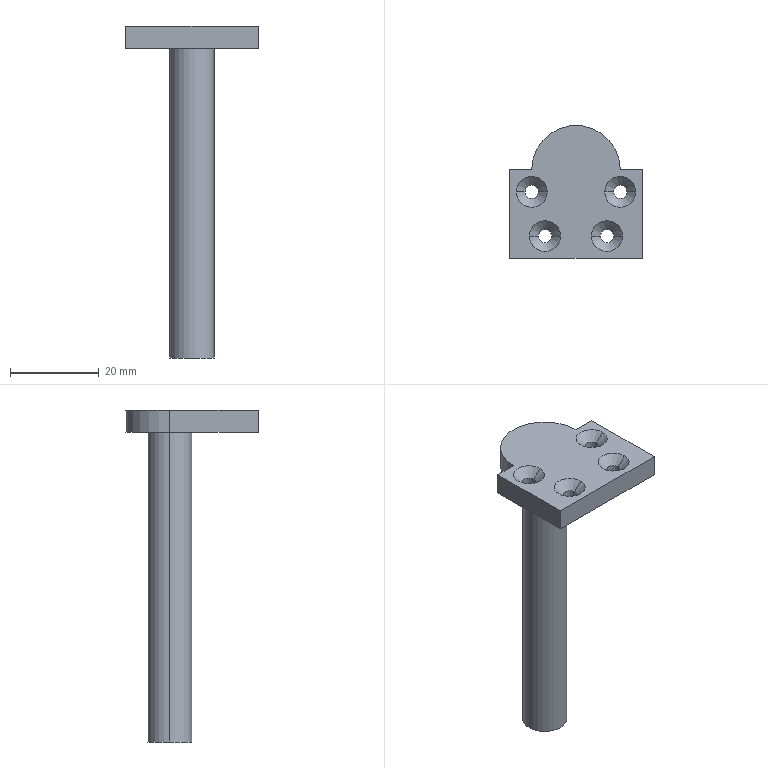Part | SolidWorks | features BaseBody 1 | 1 solid | 27 faces | box 30 x 30 x 75 mm | volume 9033 mm3 | cylinder 11 | cone 8 | plane 8 | commonest cylinder face diameters 3 x8 10 x2 20 x1
STEP:
#1=CARTESIAN_POINT('',(8.5,-5.,-2.));
#2=VERTEX_POINT('',#1);
#3=CARTESIAN_POINT('',(11.5,-5.,-2.));
#4=VERTEX_POINT('',#3);
#5=CARTESIAN_POINT('',(10.,-5.,-2.));
#6=DIRECTION('',(0.,0.,-1.));
#7=DIRECTION('',(-1.,0.,0.));
#8=AXIS2_PLACEMENT_3D('',#5,#6,#7);
#9=CIRCLE('',#8,1.5);
#10=EDGE_CURVE('',#2,#4,#9,.T.);
#11=ORIENTED_EDGE('',*,*,#10,.T.);
#12=CARTESIAN_POINT('',(13.5,-5.,0.));
#13=VERTEX_POINT('',#12);
#14=CARTESIAN_POINT('',(12.5,-5.,-1.));
#15=DIRECTION('',(0.7071,0.,0.7071));
#16=VECTOR('',#15,1000.);
#17=LINE('',#14,#16);
#18=EDGE_CURVE('',#4,#13,#17,.T.);
#19=ORIENTED_EDGE('',*,*,#18,.T.);
#20=CARTESIAN_POINT('',(6.5,-5.,0.));
#21=VERTEX_POINT('',#20);
#22=CARTESIAN_POINT('',(10.,-5.,0.));
#23=DIRECTION('',(0.,0.,1.));
#24=DIRECTION('',(-1.,0.,0.));
#25=AXIS2_PLACEMENT_3D('',#22,#23,#24);
#26=CIRCLE('',#25,3.5);
#27=EDGE_CURVE('',#13,#21,#26,.T.);
#28=ORIENTED_EDGE('',*,*,#27,.T.);
#29=CARTESIAN_POINT('',(7.5,-5.,-1.));
#30=DIRECTION('',(-0.7071,0.,0.7071));
#31=VECTOR('',#30,1000.);
#32=LINE('',#29,#31);
#33=EDGE_CURVE('',#2,#21,#32,.T.);
#34=ORIENTED_EDGE('',*,*,#33,.F.);
#35=EDGE_LOOP('',(#11,#19,#28,#34));
#36=FACE_OUTER_BOUND('',#35,.T.);
#37=CARTESIAN_POINT('',(10.,-5.,-1.));
#38=DIRECTION('',(0.,0.,1.));
#39=DIRECTION('',(-1.,0.,0.));
#40=AXIS2_PLACEMENT_3D('',#37,#38,#39);
#41=CONICAL_SURFACE('',#40,2.5,0.7854);
#42=ADVANCED_FACE('',(#36),#41,.F.);
#43=CARTESIAN_POINT('',(11.5,-5.,-5.));
#44=VERTEX_POINT('',#43);
#45=CARTESIAN_POINT('',(8.5,-5.,-5.));
#46=VERTEX_POINT('',#45);
#47=CARTESIAN_POINT('',(10.,-5.,-5.));
#48=DIRECTION('',(0.,0.,1.));
#49=DIRECTION('',(-1.,0.,0.));
#50=AXIS2_PLACEMENT_3D('',#47,#48,#49);
#51=CIRCLE('',#50,1.5);
#52=EDGE_CURVE('',#44,#46,#51,.T.);
#53=ORIENTED_EDGE('',*,*,#52,.F.);
#54=CARTESIAN_POINT('',(11.5,-5.,0.));
#55=DIRECTION('',(0.,0.,1.));
#56=VECTOR('',#55,1000.);
#57=LINE('',#54,#56);
#58=EDGE_CURVE('',#44,#4,#57,.T.);
#59=ORIENTED_EDGE('',*,*,#58,.T.);
#60=ORIENTED_EDGE('',*,*,#10,.F.);
#61=CARTESIAN_POINT('',(8.5,-5.,0.));
#62=DIRECTION('',(0.,0.,1.));
#63=VECTOR('',#62,1000.);
#64=LINE('',#61,#63);
#65=EDGE_CURVE('',#46,#2,#64,.T.);
#66=ORIENTED_EDGE('',*,*,#65,.F.);
#67=EDGE_LOOP('',(#53,#59,#60,#66));
#68=FACE_OUTER_BOUND('',#67,.T.);
#69=CARTESIAN_POINT('',(10.,-5.,0.));
#70=DIRECTION('',(0.,0.,1.));
#71=DIRECTION('',(-1.,0.,0.));
#72=AXIS2_PLACEMENT_3D('',#69,#70,#71);
#73=CYLINDRICAL_SURFACE('',#72,1.5);
#74=ADVANCED_FACE('',(#68),#73,.F.);
#75=CARTESIAN_POINT('',(5.5,-15.,-2.));
#76=VERTEX_POINT('',#75);
#77=CARTESIAN_POINT('',(8.5,-15.,-2.));
#78=VERTEX_POINT('',#77);
#79=CARTESIAN_POINT('',(7.,-15.,-2.));
#80=DIRECTION('',(0.,0.,-1.));
#81=DIRECTION('',(-1.,0.,0.));
#82=AXIS2_PLACEMENT_3D('',#79,#80,#81);
#83=CIRCLE('',#82,1.5);
#84=EDGE_CURVE('',#76,#78,#83,.T.);
#85=ORIENTED_EDGE('',*,*,#84,.T.);
#86=CARTESIAN_POINT('',(10.5,-15.,0.));
#87=VERTEX_POINT('',#86);
#88=CARTESIAN_POINT('',(9.5,-15.,-1.));
#89=DIRECTION('',(0.7071,0.,0.7071));
#90=VECTOR('',#89,1000.);
#91=LINE('',#88,#90);
#92=EDGE_CURVE('',#78,#87,#91,.T.);
#93=ORIENTED_EDGE('',*,*,#92,.T.);
#94=CARTESIAN_POINT('',(3.5,-15.,0.));
#95=VERTEX_POINT('',#94);
#96=CARTESIAN_POINT('',(7.,-15.,0.));
#97=DIRECTION('',(0.,0.,1.));
#98=DIRECTION('',(-1.,0.,0.));
#99=AXIS2_PLACEMENT_3D('',#96,#97,#98);
#100=CIRCLE('',#99,3.5);
#101=EDGE_CURVE('',#87,#95,#100,.T.);
#102=ORIENTED_EDGE('',*,*,#101,.T.);
#103=CARTESIAN_POINT('',(4.5,-15.,-1.));
#104=DIRECTION('',(-0.7071,0.,0.7071));
#105=VECTOR('',#104,1000.);
#106=LINE('',#103,#105);
#107=EDGE_CURVE('',#76,#95,#106,.T.);
#108=ORIENTED_EDGE('',*,*,#107,.F.);
#109=EDGE_LOOP('',(#85,#93,#102,#108));
#110=FACE_OUTER_BOUND('',#109,.T.);
#111=CARTESIAN_POINT('',(7.,-15.,-1.));
#112=DIRECTION('',(0.,0.,1.));
#113=DIRECTION('',(-1.,0.,0.));
#114=AXIS2_PLACEMENT_3D('',#111,#112,#113);
#115=CONICAL_SURFACE('',#114,2.5,0.7854);
#116=ADVANCED_FACE('',(#110),#115,.F.);
#117=CARTESIAN_POINT('',(8.5,-15.,-5.));
#118=VERTEX_POINT('',#117);
#119=CARTESIAN_POINT('',(5.5,-15.,-5.));
#120=VERTEX_POINT('',#119);
#121=CARTESIAN_POINT('',(7.,-15.,-5.));
#122=DIRECTION('',(0.,0.,1.));
#123=DIRECTION('',(-1.,0.,0.));
#124=AXIS2_PLACEMENT_3D('',#121,#122,#123);
#125=CIRCLE('',#124,1.5);
#126=EDGE_CURVE('',#118,#120,#125,.T.);
#127=ORIENTED_EDGE('',*,*,#126,.F.);
#128=CARTESIAN_POINT('',(8.5,-15.,0.));
#129=DIRECTION('',(0.,0.,1.));
#130=VECTOR('',#129,1000.);
#131=LINE('',#128,#130);
#132=EDGE_CURVE('',#118,#78,#131,.T.);
#133=ORIENTED_EDGE('',*,*,#132,.T.);
#134=ORIENTED_EDGE('',*,*,#84,.F.);
#135=CARTESIAN_POINT('',(5.5,-15.,0.));
#136=DIRECTION('',(0.,0.,1.));
#137=VECTOR('',#136,1000.);
#138=LINE('',#135,#137);
#139=EDGE_CURVE('',#120,#76,#138,.T.);
#140=ORIENTED_EDGE('',*,*,#139,.F.);
#141=EDGE_LOOP('',(#127,#133,#134,#140));
#142=FACE_OUTER_BOUND('',#141,.T.);
#143=CARTESIAN_POINT('',(7.,-15.,0.));
#144=DIRECTION('',(0.,0.,1.));
#145=DIRECTION('',(-1.,0.,0.));
#146=AXIS2_PLACEMENT_3D('',#143,#144,#145);
#147=CYLINDRICAL_SURFACE('',#146,1.5);
#148=ADVANCED_FACE('',(#142),#147,.F.);
#149=CARTESIAN_POINT('',(-8.5,-15.,-2.));
#150=VERTEX_POINT('',#149);
#151=CARTESIAN_POINT('',(-5.5,-15.,-2.));
#152=VERTEX_POINT('',#151);
#153=CARTESIAN_POINT('',(-7.,-15.,-2.));
#154=DIRECTION('',(0.,0.,-1.));
#155=DIRECTION('',(-1.,0.,0.));
#156=AXIS2_PLACEMENT_3D('',#153,#154,#155);
#157=CIRCLE('',#156,1.5);
#158=EDGE_CURVE('',#150,#152,#157,.T.);
#159=ORIENTED_EDGE('',*,*,#158,.T.);
#160=CARTESIAN_POINT('',(-3.5,-15.,0.));
#161=VERTEX_POINT('',#160);
#162=CARTESIAN_POINT('',(-4.5,-15.,-1.));
#163=DIRECTION('',(0.7071,0.,0.7071));
#164=VECTOR('',#163,1000.);
#165=LINE('',#162,#164);
#166=EDGE_CURVE('',#152,#161,#165,.T.);
#167=ORIENTED_EDGE('',*,*,#166,.T.);
#168=CARTESIAN_POINT('',(-10.5,-15.,0.));
#169=VERTEX_POINT('',#168);
#170=CARTESIAN_POINT('',(-7.,-15.,0.));
#171=DIRECTION('',(0.,0.,1.));
#172=DIRECTION('',(-1.,0.,0.));
#173=AXIS2_PLACEMENT_3D('',#170,#171,#172);
#174=CIRCLE('',#173,3.5);
#175=EDGE_CURVE('',#161,#169,#174,.T.);
#176=ORIENTED_EDGE('',*,*,#175,.T.);
#177=CARTESIAN_POINT('',(-9.5,-15.,-1.));
#178=DIRECTION('',(-0.7071,0.,0.7071));
#179=VECTOR('',#178,1000.);
#180=LINE('',#177,#179);
#181=EDGE_CURVE('',#150,#169,#180,.T.);
#182=ORIENTED_EDGE('',*,*,#181,.F.);
#183=EDGE_LOOP('',(#159,#167,#176,#182));
#184=FACE_OUTER_BOUND('',#183,.T.);
#185=CARTESIAN_POINT('',(-7.,-15.,-1.));
#186=DIRECTION('',(0.,0.,1.));
#187=DIRECTION('',(-1.,0.,0.));
#188=AXIS2_PLACEMENT_3D('',#185,#186,#187);
#189=CONICAL_SURFACE('',#188,2.5,0.7854);
#190=ADVANCED_FACE('',(#184),#189,.F.);
#191=CARTESIAN_POINT('',(-5.5,-15.,-5.));
#192=VERTEX_POINT('',#191);
#193=CARTESIAN_POINT('',(-8.5,-15.,-5.));
#194=VERTEX_POINT('',#193);
#195=CARTESIAN_POINT('',(-7.,-15.,-5.));
#196=DIRECTION('',(0.,0.,1.));
#197=DIRECTION('',(-1.,0.,0.));
#198=AXIS2_PLACEMENT_3D('',#195,#196,#197);
#199=CIRCLE('',#198,1.5);
#200=EDGE_CURVE('',#192,#194,#199,.T.);
#201=ORIENTED_EDGE('',*,*,#200,.F.);
#202=CARTESIAN_POINT('',(-5.5,-15.,0.));
#203=DIRECTION('',(0.,0.,1.));
#204=VECTOR('',#203,1000.);
#205=LINE('',#202,#204);
#206=EDGE_CURVE('',#192,#152,#205,.T.);
#207=ORIENTED_EDGE('',*,*,#206,.T.);
#208=ORIENTED_EDGE('',*,*,#158,.F.);
#209=CARTESIAN_POINT('',(-8.5,-15.,0.));
#210=DIRECTION('',(0.,0.,1.));
#211=VECTOR('',#210,1000.);
#212=LINE('',#209,#211);
#213=EDGE_CURVE('',#194,#150,#212,.T.);
#214=ORIENTED_EDGE('',*,*,#213,.F.);
#215=EDGE_LOOP('',(#201,#207,#208,#214));
#216=FACE_OUTER_BOUND('',#215,.T.);
#217=CARTESIAN_POINT('',(-7.,-15.,0.));
#218=DIRECTION('',(0.,0.,1.));
#219=DIRECTION('',(-1.,0.,0.));
#220=AXIS2_PLACEMENT_3D('',#217,#218,#219);
#221=CYLINDRICAL_SURFACE('',#220,1.5);
#222=ADVANCED_FACE('',(#216),#221,.F.);
#223=CARTESIAN_POINT('',(-11.5,-5.,-2.));
#224=VERTEX_POINT('',#223);
#225=CARTESIAN_POINT('',(-8.5,-5.,-2.));
#226=VERTEX_POINT('',#225);
#227=CARTESIAN_POINT('',(-10.,-5.,-2.));
#228=DIRECTION('',(0.,0.,-1.));
#229=DIRECTION('',(-1.,0.,0.));
#230=AXIS2_PLACEMENT_3D('',#227,#228,#229);
#231=CIRCLE('',#230,1.5);
#232=EDGE_CURVE('',#224,#226,#231,.T.);
#233=ORIENTED_EDGE('',*,*,#232,.T.);
#234=CARTESIAN_POINT('',(-6.5,-5.,0.));
#235=VERTEX_POINT('',#234);
#236=CARTESIAN_POINT('',(-7.5,-5.,-1.));
#237=DIRECTION('',(0.7071,0.,0.7071));
#238=VECTOR('',#237,1000.);
#239=LINE('',#236,#238);
#240=EDGE_CURVE('',#226,#235,#239,.T.);
#241=ORIENTED_EDGE('',*,*,#240,.T.);
#242=CARTESIAN_POINT('',(-13.5,-5.,0.));
#243=VERTEX_POINT('',#242);
#244=CARTESIAN_POINT('',(-10.,-5.,0.));
#245=DIRECTION('',(0.,0.,1.));
#246=DIRECTION('',(-1.,0.,0.));
#247=AXIS2_PLACEMENT_3D('',#244,#245,#246);
#248=CIRCLE('',#247,3.5);
#249=EDGE_CURVE('',#235,#243,#248,.T.);
#250=ORIENTED_EDGE('',*,*,#249,.T.);
#251=CARTESIAN_POINT('',(-12.5,-5.,-1.));
#252=DIRECTION('',(-0.7071,0.,0.7071));
#253=VECTOR('',#252,1000.);
#254=LINE('',#251,#253);
#255=EDGE_CURVE('',#224,#243,#254,.T.);
#256=ORIENTED_EDGE('',*,*,#255,.F.);
#257=EDGE_LOOP('',(#233,#241,#250,#256));
#258=FACE_OUTER_BOUND('',#257,.T.);
#259=CARTESIAN_POINT('',(-10.,-5.,-1.));
#260=DIRECTION('',(0.,0.,1.));
#261=DIRECTION('',(-1.,0.,0.));
#262=AXIS2_PLACEMENT_3D('',#259,#260,#261);
#263=CONICAL_SURFACE('',#262,2.5,0.7854);
#264=ADVANCED_FACE('',(#258),#263,.F.);
#265=CARTESIAN_POINT('',(-8.5,-5.,-5.));
#266=VERTEX_POINT('',#265);
#267=CARTESIAN_POINT('',(-11.5,-5.,-5.));
#268=VERTEX_POINT('',#267);
#269=CARTESIAN_POINT('',(-10.,-5.,-5.));
#270=DIRECTION('',(0.,0.,1.));
#271=DIRECTION('',(-1.,0.,0.));
#272=AXIS2_PLACEMENT_3D('',#269,#270,#271);
#273=CIRCLE('',#272,1.5);
#274=EDGE_CURVE('',#266,#268,#273,.T.);
#275=ORIENTED_EDGE('',*,*,#274,.F.);
#276=CARTESIAN_POINT('',(-8.5,-5.,0.));
#277=DIRECTION('',(0.,0.,1.));
#278=VECTOR('',#277,1000.);
#279=LINE('',#276,#278);
#280=EDGE_CURVE('',#266,#226,#279,.T.);
#281=ORIENTED_EDGE('',*,*,#280,.T.);
#282=ORIENTED_EDGE('',*,*,#232,.F.);
#283=CARTESIAN_POINT('',(-11.5,-5.,0.));
#284=DIRECTION('',(0.,0.,1.));
#285=VECTOR('',#284,1000.);
#286=LINE('',#283,#285);
#287=EDGE_CURVE('',#268,#224,#286,.T.);
#288=ORIENTED_EDGE('',*,*,#287,.F.);
#289=EDGE_LOOP('',(#275,#281,#282,#288));
#290=FACE_OUTER_BOUND('',#289,.T.);
#291=CARTESIAN_POINT('',(-10.,-5.,0.));
#292=DIRECTION('',(0.,0.,1.));
#293=DIRECTION('',(-1.,0.,0.));
#294=AXIS2_PLACEMENT_3D('',#291,#292,#293);
#295=CYLINDRICAL_SURFACE('',#294,1.5);
#296=ADVANCED_FACE('',(#290),#295,.F.);
#297=CARTESIAN_POINT('',(-5.,0.,-75.));
#298=VERTEX_POINT('',#297);
#299=CARTESIAN_POINT('',(5.,0.,-75.));
#300=VERTEX_POINT('',#299);
#301=CARTESIAN_POINT('',(0.,0.,-75.));
#302=DIRECTION('',(0.,0.,-1.));
#303=DIRECTION('',(1.,0.,0.));
#304=AXIS2_PLACEMENT_3D('',#301,#302,#303);
#305=CIRCLE('',#304,5.);
#306=EDGE_CURVE('',#298,#300,#305,.T.);
#307=ORIENTED_EDGE('',*,*,#306,.F.);
#308=CARTESIAN_POINT('',(-5.,0.,-5.));
#309=VERTEX_POINT('',#308);
#310=CARTESIAN_POINT('',(-5.,0.,-5.));
#311=DIRECTION('',(0.,0.,1.));
#312=VECTOR('',#311,1000.);
#313=LINE('',#310,#312);
#314=EDGE_CURVE('',#298,#309,#313,.T.);
#315=ORIENTED_EDGE('',*,*,#314,.T.);
#316=CARTESIAN_POINT('',(5.,0.,-5.));
#317=VERTEX_POINT('',#316);
#318=CARTESIAN_POINT('',(0.,0.,-5.));
#319=DIRECTION('',(0.,0.,1.));
#320=DIRECTION('',(1.,0.,0.));
#321=AXIS2_PLACEMENT_3D('',#318,#319,#320);
#322=CIRCLE('',#321,5.);
#323=EDGE_CURVE('',#317,#309,#322,.T.);
#324=ORIENTED_EDGE('',*,*,#323,.F.);
#325=CARTESIAN_POINT('',(5.,0.,-5.));
#326=DIRECTION('',(0.,0.,1.));
#327=VECTOR('',#326,1000.);
#328=LINE('',#325,#327);
#329=EDGE_CURVE('',#300,#317,#328,.T.);
#330=ORIENTED_EDGE('',*,*,#329,.F.);
#331=EDGE_LOOP('',(#307,#315,#324,#330));
#332=FACE_OUTER_BOUND('',#331,.T.);
#333=CARTESIAN_POINT('',(0.,0.,-5.));
#334=DIRECTION('',(0.,0.,1.));
#335=DIRECTION('',(1.,0.,0.));
#336=AXIS2_PLACEMENT_3D('',#333,#334,#335);
#337=CYLINDRICAL_SURFACE('',#336,5.);
#338=ADVANCED_FACE('',(#332),#337,.T.);
#339=CARTESIAN_POINT('',(7.,-15.,0.));
#340=DIRECTION('',(0.,0.,1.));
#341=DIRECTION('',(-1.,0.,0.));
#342=AXIS2_PLACEMENT_3D('',#339,#340,#341);
#343=CIRCLE('',#342,3.5);
#344=EDGE_CURVE('',#95,#87,#343,.T.);
#345=ORIENTED_EDGE('',*,*,#344,.F.);
#346=ORIENTED_EDGE('',*,*,#101,.F.);
#347=EDGE_LOOP('',(#345,#346));
#348=FACE_BOUND('',#347,.T.);
#349=CARTESIAN_POINT('',(-10.,-5.,0.));
#350=DIRECTION('',(0.,0.,1.));
#351=DIRECTION('',(-1.,0.,0.));
#352=AXIS2_PLACEMENT_3D('',#349,#350,#351);
#353=CIRCLE('',#352,3.5);
#354=EDGE_CURVE('',#243,#235,#353,.T.);
#355=ORIENTED_EDGE('',*,*,#354,.F.);
#356=ORIENTED_EDGE('',*,*,#249,.F.);
#357=EDGE_LOOP('',(#355,#356));
#358=FACE_BOUND('',#357,.T.);
#359=CARTESIAN_POINT('',(-7.,-15.,0.));
#360=DIRECTION('',(0.,0.,1.));
#361=DIRECTION('',(-1.,0.,0.));
#362=AXIS2_PLACEMENT_3D('',#359,#360,#361);
#363=CIRCLE('',#362,3.5);
#364=EDGE_CURVE('',#169,#161,#363,.T.);
#365=ORIENTED_EDGE('',*,*,#364,.F.);
#366=ORIENTED_EDGE('',*,*,#175,.F.);
#367=EDGE_LOOP('',(#365,#366));
#368=FACE_BOUND('',#367,.T.);
#369=CARTESIAN_POINT('',(10.,-5.,0.));
#370=DIRECTION('',(0.,0.,1.));
#371=DIRECTION('',(-1.,0.,0.));
#372=AXIS2_PLACEMENT_3D('',#369,#370,#371);
#373=CIRCLE('',#372,3.5);
#374=EDGE_CURVE('',#21,#13,#373,.T.);
#375=ORIENTED_EDGE('',*,*,#374,.F.);
#376=ORIENTED_EDGE('',*,*,#27,.F.);
#377=EDGE_LOOP('',(#375,#376));
#378=FACE_BOUND('',#377,.T.);
#379=CARTESIAN_POINT('',(10.,0.,0.));
#380=VERTEX_POINT('',#379);
#381=CARTESIAN_POINT('',(-10.,0.,0.));
#382=VERTEX_POINT('',#381);
#383=CARTESIAN_POINT('',(0.,0.,0.));
#384=DIRECTION('',(0.,0.,1.));
#385=DIRECTION('',(1.,0.,0.));
#386=AXIS2_PLACEMENT_3D('',#383,#384,#385);
#387=CIRCLE('',#386,10.);
#388=EDGE_CURVE('',#380,#382,#387,.T.);
#389=ORIENTED_EDGE('',*,*,#388,.T.);
#390=CARTESIAN_POINT('',(-15.,0.,0.));
#391=VERTEX_POINT('',#390);
#392=CARTESIAN_POINT('',(15.,0.,0.));
#393=DIRECTION('',(-1.,0.,0.));
#394=VECTOR('',#393,1000.);
#395=LINE('',#392,#394);
#396=EDGE_CURVE('',#382,#391,#395,.T.);
#397=ORIENTED_EDGE('',*,*,#396,.T.);
#398=CARTESIAN_POINT('',(-15.,-20.,0.));
#399=VERTEX_POINT('',#398);
#400=CARTESIAN_POINT('',(-15.,0.,0.));
#401=DIRECTION('',(0.,-1.,0.));
#402=VECTOR('',#401,1000.);
#403=LINE('',#400,#402);
#404=EDGE_CURVE('',#391,#399,#403,.T.);
#405=ORIENTED_EDGE('',*,*,#404,.T.);
#406=CARTESIAN_POINT('',(15.,-20.,0.));
#407=VERTEX_POINT('',#406);
#408=CARTESIAN_POINT('',(-15.,-20.,0.));
#409=DIRECTION('',(1.,0.,0.));
#410=VECTOR('',#409,1000.);
#411=LINE('',#408,#410);
#412=EDGE_CURVE('',#399,#407,#411,.T.);
#413=ORIENTED_EDGE('',*,*,#412,.T.);
#414=CARTESIAN_POINT('',(15.,0.,0.));
#415=VERTEX_POINT('',#414);
#416=CARTESIAN_POINT('',(15.,-20.,0.));
#417=DIRECTION('',(0.,1.,0.));
#418=VECTOR('',#417,1000.);
#419=LINE('',#416,#418);
#420=EDGE_CURVE('',#407,#415,#419,.T.);
#421=ORIENTED_EDGE('',*,*,#420,.T.);
#422=CARTESIAN_POINT('',(15.,0.,0.));
#423=DIRECTION('',(-1.,0.,0.));
#424=VECTOR('',#423,1000.);
#425=LINE('',#422,#424);
#426=EDGE_CURVE('',#415,#380,#425,.T.);
#427=ORIENTED_EDGE('',*,*,#426,.T.);
#428=EDGE_LOOP('',(#389,#397,#405,#413,#421,#427));
#429=FACE_OUTER_BOUND('',#428,.T.);
#430=CARTESIAN_POINT('',(0.,3.443,0.));
#431=DIRECTION('',(0.,0.,1.));
#432=DIRECTION('',(1.,0.,0.));
#433=AXIS2_PLACEMENT_3D('',#430,#431,#432);
#434=PLANE('',#433);
#435=ADVANCED_FACE('',(#348,#358,#368,#378,#429),#434,.T.);
#436=CARTESIAN_POINT('',(0.,0.,-75.));
#437=DIRECTION('',(0.,0.,-1.));
#438=DIRECTION('',(1.,0.,0.));
#439=AXIS2_PLACEMENT_3D('',#436,#437,#438);
#440=CIRCLE('',#439,5.);
#441=EDGE_CURVE('',#300,#298,#440,.T.);
#442=ORIENTED_EDGE('',*,*,#441,.T.);
#443=ORIENTED_EDGE('',*,*,#306,.T.);
#444=EDGE_LOOP('',(#442,#443));
#445=FACE_OUTER_BOUND('',#444,.T.);
#446=CARTESIAN_POINT('',(0.,0.,-75.));
#447=DIRECTION('',(0.,0.,1.));
#448=DIRECTION('',(1.,0.,0.));
#449=AXIS2_PLACEMENT_3D('',#446,#447,#448);
#450=PLANE('',#449);
#451=ADVANCED_FACE('',(#445),#450,.F.);
#452=CARTESIAN_POINT('',(-10.,0.,-5.));
#453=VERTEX_POINT('',#452);
#454=CARTESIAN_POINT('',(-10.,0.,0.));
#455=DIRECTION('',(0.,0.,-1.));
#456=VECTOR('',#455,1000.);
#457=LINE('',#454,#456);
#458=EDGE_CURVE('',#382,#453,#457,.T.);
#459=ORIENTED_EDGE('',*,*,#458,.T.);
#460=CARTESIAN_POINT('',(-15.,0.,-5.));
#461=VERTEX_POINT('',#460);
#462=CARTESIAN_POINT('',(15.,0.,-5.));
#463=DIRECTION('',(1.,0.,0.));
#464=VECTOR('',#463,1000.);
#465=LINE('',#462,#464);
#466=EDGE_CURVE('',#461,#453,#465,.T.);
#467=ORIENTED_EDGE('',*,*,#466,.F.);
#468=CARTESIAN_POINT('',(-15.,0.,0.));
#469=DIRECTION('',(0.,0.,-1.));
#470=VECTOR('',#469,1000.);
#471=LINE('',#468,#470);
#472=EDGE_CURVE('',#391,#461,#471,.T.);
#473=ORIENTED_EDGE('',*,*,#472,.F.);
#474=ORIENTED_EDGE('',*,*,#396,.F.);
#475=EDGE_LOOP('',(#459,#467,#473,#474));
#476=FACE_OUTER_BOUND('',#475,.T.);
#477=CARTESIAN_POINT('',(-15.,0.,0.));
#478=DIRECTION('',(0.,1.,0.));
#479=DIRECTION('',(1.,0.,0.));
#480=AXIS2_PLACEMENT_3D('',#477,#478,#479);
#481=PLANE('',#480);
#482=ADVANCED_FACE('',(#476),#481,.T.);
#483=CARTESIAN_POINT('',(10.,0.,-5.));
#484=VERTEX_POINT('',#483);
#485=CARTESIAN_POINT('',(10.,0.,0.));
#486=DIRECTION('',(0.,0.,-1.));
#487=VECTOR('',#486,1000.);
#488=LINE('',#485,#487);
#489=EDGE_CURVE('',#380,#484,#488,.T.);
#490=ORIENTED_EDGE('',*,*,#489,.F.);
#491=ORIENTED_EDGE('',*,*,#426,.F.);
#492=CARTESIAN_POINT('',(15.,0.,-5.));
#493=VERTEX_POINT('',#492);
#494=CARTESIAN_POINT('',(15.,0.,0.));
#495=DIRECTION('',(0.,0.,-1.));
#496=VECTOR('',#495,1000.);
#497=LINE('',#494,#496);
#498=EDGE_CURVE('',#415,#493,#497,.T.);
#499=ORIENTED_EDGE('',*,*,#498,.T.);
#500=CARTESIAN_POINT('',(15.,0.,-5.));
#501=DIRECTION('',(1.,0.,0.));
#502=VECTOR('',#501,1000.);
#503=LINE('',#500,#502);
#504=EDGE_CURVE('',#484,#493,#503,.T.);
#505=ORIENTED_EDGE('',*,*,#504,.F.);
#506=EDGE_LOOP('',(#490,#491,#499,#505));
#507=FACE_OUTER_BOUND('',#506,.T.);
#508=CARTESIAN_POINT('',(-15.,0.,0.));
#509=DIRECTION('',(0.,1.,0.));
#510=DIRECTION('',(1.,0.,0.));
#511=AXIS2_PLACEMENT_3D('',#508,#509,#510);
#512=PLANE('',#511);
#513=ADVANCED_FACE('',(#507),#512,.T.);
#514=ORIENTED_EDGE('',*,*,#412,.F.);
#515=CARTESIAN_POINT('',(-15.,-20.,-5.));
#516=VERTEX_POINT('',#515);
#517=CARTESIAN_POINT('',(-15.,-20.,0.));
#518=DIRECTION('',(0.,0.,-1.));
#519=VECTOR('',#518,1000.);
#520=LINE('',#517,#519);
#521=EDGE_CURVE('',#399,#516,#520,.T.);
#522=ORIENTED_EDGE('',*,*,#521,.T.);
#523=CARTESIAN_POINT('',(15.,-20.,-5.));
#524=VERTEX_POINT('',#523);
#525=CARTESIAN_POINT('',(-15.,-20.,-5.));
#526=DIRECTION('',(-1.,0.,0.));
#527=VECTOR('',#526,1000.);
#528=LINE('',#525,#527);
#529=EDGE_CURVE('',#524,#516,#528,.T.);
#530=ORIENTED_EDGE('',*,*,#529,.F.);
#531=CARTESIAN_POINT('',(15.,-20.,0.));
#532=DIRECTION('',(0.,0.,-1.));
#533=VECTOR('',#532,1000.);
#534=LINE('',#531,#533);
#535=EDGE_CURVE('',#407,#524,#534,.T.);
#536=ORIENTED_EDGE('',*,*,#535,.F.);
#537=EDGE_LOOP('',(#514,#522,#530,#536));
#538=FACE_OUTER_BOUND('',#537,.T.);
#539=CARTESIAN_POINT('',(15.,-20.,0.));
#540=DIRECTION('',(0.,-1.,0.));
#541=DIRECTION('',(-1.,0.,0.));
#542=AXIS2_PLACEMENT_3D('',#539,#540,#541);
#543=PLANE('',#542);
#544=ADVANCED_FACE('',(#538),#543,.T.);
#545=ORIENTED_EDGE('',*,*,#420,.F.);
#546=ORIENTED_EDGE('',*,*,#535,.T.);
#547=CARTESIAN_POINT('',(15.,-20.,-5.));
#548=DIRECTION('',(0.,-1.,0.));
#549=VECTOR('',#548,1000.);
#550=LINE('',#547,#549);
#551=EDGE_CURVE('',#493,#524,#550,.T.);
#552=ORIENTED_EDGE('',*,*,#551,.F.);
#553=ORIENTED_EDGE('',*,*,#498,.F.);
#554=EDGE_LOOP('',(#545,#546,#552,#553));
#555=FACE_OUTER_BOUND('',#554,.T.);
#556=CARTESIAN_POINT('',(15.,0.,0.));
#557=DIRECTION('',(1.,0.,0.));
#558=DIRECTION('',(0.,1.,0.));
#559=AXIS2_PLACEMENT_3D('',#556,#557,#558);
#560=PLANE('',#559);
#561=ADVANCED_FACE('',(#555),#560,.T.);
#562=ORIENTED_EDGE('',*,*,#404,.F.);
#563=ORIENTED_EDGE('',*,*,#472,.T.);
#564=CARTESIAN_POINT('',(-15.,0.,-5.));
#565=DIRECTION('',(0.,1.,0.));
#566=VECTOR('',#565,1000.);
#567=LINE('',#564,#566);
#568=EDGE_CURVE('',#516,#461,#567,.T.);
#569=ORIENTED_EDGE('',*,*,#568,.F.);
#570=ORIENTED_EDGE('',*,*,#521,.F.);
#571=EDGE_LOOP('',(#562,#563,#569,#570));
#572=FACE_OUTER_BOUND('',#571,.T.);
#573=CARTESIAN_POINT('',(-15.,-20.,0.));
#574=DIRECTION('',(-1.,0.,0.));
#575=DIRECTION('',(0.,0.,1.));
#576=AXIS2_PLACEMENT_3D('',#573,#574,#575);
#577=PLANE('',#576);
#578=ADVANCED_FACE('',(#572),#577,.T.);
#579=ORIENTED_EDGE('',*,*,#388,.F.);
#580=ORIENTED_EDGE('',*,*,#489,.T.);
#581=CARTESIAN_POINT('',(0.,0.,-5.));
#582=DIRECTION('',(0.,0.,-1.));
#583=DIRECTION('',(1.,0.,0.));
#584=AXIS2_PLACEMENT_3D('',#581,#582,#583);
#585=CIRCLE('',#584,10.);
#586=EDGE_CURVE('',#453,#484,#585,.T.);
#587=ORIENTED_EDGE('',*,*,#586,.F.);
#588=ORIENTED_EDGE('',*,*,#458,.F.);
#589=EDGE_LOOP('',(#579,#580,#587,#588));
#590=FACE_OUTER_BOUND('',#589,.T.);
#591=CARTESIAN_POINT('',(0.,0.,0.));
#592=DIRECTION('',(0.,0.,1.));
#593=DIRECTION('',(1.,0.,0.));
#594=AXIS2_PLACEMENT_3D('',#591,#592,#593);
#595=CYLINDRICAL_SURFACE('',#594,10.);
#596=ADVANCED_FACE('',(#590),#595,.T.);
#597=ORIENTED_EDGE('',*,*,#323,.T.);
#598=CARTESIAN_POINT('',(0.,0.,-5.));
#599=DIRECTION('',(0.,0.,1.));
#600=DIRECTION('',(1.,0.,0.));
#601=AXIS2_PLACEMENT_3D('',#598,#599,#600);
#602=CIRCLE('',#601,5.);
#603=EDGE_CURVE('',#309,#317,#602,.T.);
#604=ORIENTED_EDGE('',*,*,#603,.T.);
#605=EDGE_LOOP('',(#597,#604));
#606=FACE_BOUND('',#605,.T.);
#607=CARTESIAN_POINT('',(-7.,-15.,-5.));
#608=DIRECTION('',(0.,0.,1.));
#609=DIRECTION('',(-1.,0.,0.));
#610=AXIS2_PLACEMENT_3D('',#607,#608,#609);
#611=CIRCLE('',#610,1.5);
#612=EDGE_CURVE('',#194,#192,#611,.T.);
#613=ORIENTED_EDGE('',*,*,#612,.T.);
#614=ORIENTED_EDGE('',*,*,#200,.T.);
#615=EDGE_LOOP('',(#613,#614));
#616=FACE_BOUND('',#615,.T.);
#617=CARTESIAN_POINT('',(-10.,-5.,-5.));
#618=DIRECTION('',(0.,0.,1.));
#619=DIRECTION('',(-1.,0.,0.));
#620=AXIS2_PLACEMENT_3D('',#617,#618,#619);
#621=CIRCLE('',#620,1.5);
#622=EDGE_CURVE('',#268,#266,#621,.T.);
#623=ORIENTED_EDGE('',*,*,#622,.T.);
#624=ORIENTED_EDGE('',*,*,#274,.T.);
#625=EDGE_LOOP('',(#623,#624));
#626=FACE_BOUND('',#625,.T.);
#627=CARTESIAN_POINT('',(7.,-15.,-5.));
#628=DIRECTION('',(0.,0.,1.));
#629=DIRECTION('',(-1.,0.,0.));
#630=AXIS2_PLACEMENT_3D('',#627,#628,#629);
#631=CIRCLE('',#630,1.5);
#632=EDGE_CURVE('',#120,#118,#631,.T.);
#633=ORIENTED_EDGE('',*,*,#632,.T.);
#634=ORIENTED_EDGE('',*,*,#126,.T.);
#635=EDGE_LOOP('',(#633,#634));
#636=FACE_BOUND('',#635,.T.);
#637=CARTESIAN_POINT('',(10.,-5.,-5.));
#638=DIRECTION('',(0.,0.,1.));
#639=DIRECTION('',(-1.,0.,0.));
#640=AXIS2_PLACEMENT_3D('',#637,#638,#639);
#641=CIRCLE('',#640,1.5);
#642=EDGE_CURVE('',#46,#44,#641,.T.);
#643=ORIENTED_EDGE('',*,*,#642,.T.);
#644=ORIENTED_EDGE('',*,*,#52,.T.);
#645=EDGE_LOOP('',(#643,#644));
#646=FACE_BOUND('',#645,.T.);
#647=ORIENTED_EDGE('',*,*,#586,.T.);
#648=ORIENTED_EDGE('',*,*,#504,.T.);
#649=ORIENTED_EDGE('',*,*,#551,.T.);
#650=ORIENTED_EDGE('',*,*,#529,.T.);
#651=ORIENTED_EDGE('',*,*,#568,.T.);
#652=ORIENTED_EDGE('',*,*,#466,.T.);
#653=EDGE_LOOP('',(#647,#648,#649,#650,#651,#652));
#654=FACE_OUTER_BOUND('',#653,.T.);
#655=CARTESIAN_POINT('',(0.,3.443,-5.));
#656=DIRECTION('',(0.,0.,1.));
#657=DIRECTION('',(1.,0.,0.));
#658=AXIS2_PLACEMENT_3D('',#655,#656,#657);
#659=PLANE('',#658);
#660=ADVANCED_FACE('',(#606,#616,#626,#636,#646,#654),#659,.F.);
#661=ORIENTED_EDGE('',*,*,#314,.F.);
#662=ORIENTED_EDGE('',*,*,#441,.F.);
#663=ORIENTED_EDGE('',*,*,#329,.T.);
#664=ORIENTED_EDGE('',*,*,#603,.F.);
#665=EDGE_LOOP('',(#661,#662,#663,#664));
#666=FACE_OUTER_BOUND('',#665,.T.);
#667=CARTESIAN_POINT('',(0.,0.,-5.));
#668=DIRECTION('',(0.,0.,1.));
#669=DIRECTION('',(1.,0.,0.));
#670=AXIS2_PLACEMENT_3D('',#667,#668,#669);
#671=CYLINDRICAL_SURFACE('',#670,5.);
#672=ADVANCED_FACE('',(#666),#671,.T.);
#673=ORIENTED_EDGE('',*,*,#280,.F.);
#674=ORIENTED_EDGE('',*,*,#622,.F.);
#675=ORIENTED_EDGE('',*,*,#287,.T.);
#676=CARTESIAN_POINT('',(-10.,-5.,-2.));
#677=DIRECTION('',(0.,0.,-1.));
#678=DIRECTION('',(-1.,0.,0.));
#679=AXIS2_PLACEMENT_3D('',#676,#677,#678);
#680=CIRCLE('',#679,1.5);
#681=EDGE_CURVE('',#226,#224,#680,.T.);
#682=ORIENTED_EDGE('',*,*,#681,.F.);
#683=EDGE_LOOP('',(#673,#674,#675,#682));
#684=FACE_OUTER_BOUND('',#683,.T.);
#685=CARTESIAN_POINT('',(-10.,-5.,0.));
#686=DIRECTION('',(0.,0.,1.));
#687=DIRECTION('',(-1.,0.,0.));
#688=AXIS2_PLACEMENT_3D('',#685,#686,#687);
#689=CYLINDRICAL_SURFACE('',#688,1.5);
#690=ADVANCED_FACE('',(#684),#689,.F.);
#691=ORIENTED_EDGE('',*,*,#240,.F.);
#692=ORIENTED_EDGE('',*,*,#681,.T.);
#693=ORIENTED_EDGE('',*,*,#255,.T.);
#694=ORIENTED_EDGE('',*,*,#354,.T.);
#695=EDGE_LOOP('',(#691,#692,#693,#694));
#696=FACE_OUTER_BOUND('',#695,.T.);
#697=CARTESIAN_POINT('',(-10.,-5.,-1.));
#698=DIRECTION('',(0.,0.,1.));
#699=DIRECTION('',(-1.,0.,0.));
#700=AXIS2_PLACEMENT_3D('',#697,#698,#699);
#701=CONICAL_SURFACE('',#700,2.5,0.7854);
#702=ADVANCED_FACE('',(#696),#701,.F.);
#703=ORIENTED_EDGE('',*,*,#206,.F.);
#704=ORIENTED_EDGE('',*,*,#612,.F.);
#705=ORIENTED_EDGE('',*,*,#213,.T.);
#706=CARTESIAN_POINT('',(-7.,-15.,-2.));
#707=DIRECTION('',(0.,0.,-1.));
#708=DIRECTION('',(-1.,0.,0.));
#709=AXIS2_PLACEMENT_3D('',#706,#707,#708);
#710=CIRCLE('',#709,1.5);
#711=EDGE_CURVE('',#152,#150,#710,.T.);
#712=ORIENTED_EDGE('',*,*,#711,.F.);
#713=EDGE_LOOP('',(#703,#704,#705,#712));
#714=FACE_OUTER_BOUND('',#713,.T.);
#715=CARTESIAN_POINT('',(-7.,-15.,0.));
#716=DIRECTION('',(0.,0.,1.));
#717=DIRECTION('',(-1.,0.,0.));
#718=AXIS2_PLACEMENT_3D('',#715,#716,#717);
#719=CYLINDRICAL_SURFACE('',#718,1.5);
#720=ADVANCED_FACE('',(#714),#719,.F.);
#721=ORIENTED_EDGE('',*,*,#166,.F.);
#722=ORIENTED_EDGE('',*,*,#711,.T.);
#723=ORIENTED_EDGE('',*,*,#181,.T.);
#724=ORIENTED_EDGE('',*,*,#364,.T.);
#725=EDGE_LOOP('',(#721,#722,#723,#724));
#726=FACE_OUTER_BOUND('',#725,.T.);
#727=CARTESIAN_POINT('',(-7.,-15.,-1.));
#728=DIRECTION('',(0.,0.,1.));
#729=DIRECTION('',(-1.,0.,0.));
#730=AXIS2_PLACEMENT_3D('',#727,#728,#729);
#731=CONICAL_SURFACE('',#730,2.5,0.7854);
#732=ADVANCED_FACE('',(#726),#731,.F.);
#733=ORIENTED_EDGE('',*,*,#132,.F.);
#734=ORIENTED_EDGE('',*,*,#632,.F.);
#735=ORIENTED_EDGE('',*,*,#139,.T.);
#736=CARTESIAN_POINT('',(7.,-15.,-2.));
#737=DIRECTION('',(0.,0.,-1.));
#738=DIRECTION('',(-1.,0.,0.));
#739=AXIS2_PLACEMENT_3D('',#736,#737,#738);
#740=CIRCLE('',#739,1.5);
#741=EDGE_CURVE('',#78,#76,#740,.T.);
#742=ORIENTED_EDGE('',*,*,#741,.F.);
#743=EDGE_LOOP('',(#733,#734,#735,#742));
#744=FACE_OUTER_BOUND('',#743,.T.);
#745=CARTESIAN_POINT('',(7.,-15.,0.));
#746=DIRECTION('',(0.,0.,1.));
#747=DIRECTION('',(-1.,0.,0.));
#748=AXIS2_PLACEMENT_3D('',#745,#746,#747);
#749=CYLINDRICAL_SURFACE('',#748,1.5);
#750=ADVANCED_FACE('',(#744),#749,.F.);
#751=ORIENTED_EDGE('',*,*,#92,.F.);
#752=ORIENTED_EDGE('',*,*,#741,.T.);
#753=ORIENTED_EDGE('',*,*,#107,.T.);
#754=ORIENTED_EDGE('',*,*,#344,.T.);
#755=EDGE_LOOP('',(#751,#752,#753,#754));
#756=FACE_OUTER_BOUND('',#755,.T.);
#757=CARTESIAN_POINT('',(7.,-15.,-1.));
#758=DIRECTION('',(0.,0.,1.));
#759=DIRECTION('',(-1.,0.,0.));
#760=AXIS2_PLACEMENT_3D('',#757,#758,#759);
#761=CONICAL_SURFACE('',#760,2.5,0.7854);
#762=ADVANCED_FACE('',(#756),#761,.F.);
#763=ORIENTED_EDGE('',*,*,#58,.F.);
#764=ORIENTED_EDGE('',*,*,#642,.F.);
#765=ORIENTED_EDGE('',*,*,#65,.T.);
#766=CARTESIAN_POINT('',(10.,-5.,-2.));
#767=DIRECTION('',(0.,0.,-1.));
#768=DIRECTION('',(-1.,0.,0.));
#769=AXIS2_PLACEMENT_3D('',#766,#767,#768);
#770=CIRCLE('',#769,1.5);
#771=EDGE_CURVE('',#4,#2,#770,.T.);
#772=ORIENTED_EDGE('',*,*,#771,.F.);
#773=EDGE_LOOP('',(#763,#764,#765,#772));
#774=FACE_OUTER_BOUND('',#773,.T.);
#775=CARTESIAN_POINT('',(10.,-5.,0.));
#776=DIRECTION('',(0.,0.,1.));
#777=DIRECTION('',(-1.,0.,0.));
#778=AXIS2_PLACEMENT_3D('',#775,#776,#777);
#779=CYLINDRICAL_SURFACE('',#778,1.5);
#780=ADVANCED_FACE('',(#774),#779,.F.);
#781=ORIENTED_EDGE('',*,*,#18,.F.);
#782=ORIENTED_EDGE('',*,*,#771,.T.);
#783=ORIENTED_EDGE('',*,*,#33,.T.);
#784=ORIENTED_EDGE('',*,*,#374,.T.);
#785=EDGE_LOOP('',(#781,#782,#783,#784));
#786=FACE_OUTER_BOUND('',#785,.T.);
#787=CARTESIAN_POINT('',(10.,-5.,-1.));
#788=DIRECTION('',(0.,0.,1.));
#789=DIRECTION('',(-1.,0.,0.));
#790=AXIS2_PLACEMENT_3D('',#787,#788,#789);
#791=CONICAL_SURFACE('',#790,2.5,0.7854);
#792=ADVANCED_FACE('',(#786),#791,.F.);
#793=CLOSED_SHELL('',(#42,#74,#116,#148,#190,#222,#264,#296,#338,#435,#451,#482,#513,#544,#561,#578,#596,#660,#672,#690,#702,#720,#732,#750,#762,#780,#792));
#794=MANIFOLD_SOLID_BREP('',#793);
#795=CARTESIAN_POINT('',(0.,0.,0.));
#796=DIRECTION('',(0.,0.,1.));
#797=DIRECTION('',(1.,0.,0.));
#798=AXIS2_PLACEMENT_3D('',#795,#796,#797);
#799=(LENGTH_UNIT()NAMED_UNIT(*)SI_UNIT(.MILLI.,.METRE.));
#800=UNCERTAINTY_MEASURE_WITH_UNIT(LENGTH_MEASURE(0.00001),#799,'','');
#801=(NAMED_UNIT(*)PLANE_ANGLE_UNIT()SI_UNIT($,.RADIAN.));
#802=(NAMED_UNIT(*)SI_UNIT($,.STERADIAN.)SOLID_ANGLE_UNIT());
#803=(GEOMETRIC_REPRESENTATION_CONTEXT(3)GLOBAL_UNCERTAINTY_ASSIGNED_CONTEXT((#800))GLOBAL_UNIT_ASSIGNED_CONTEXT((#799,#801,#802))REPRESENTATION_CONTEXT('',''));
#804=ADVANCED_BREP_SHAPE_REPRESENTATION('',(#794,#798),#803);